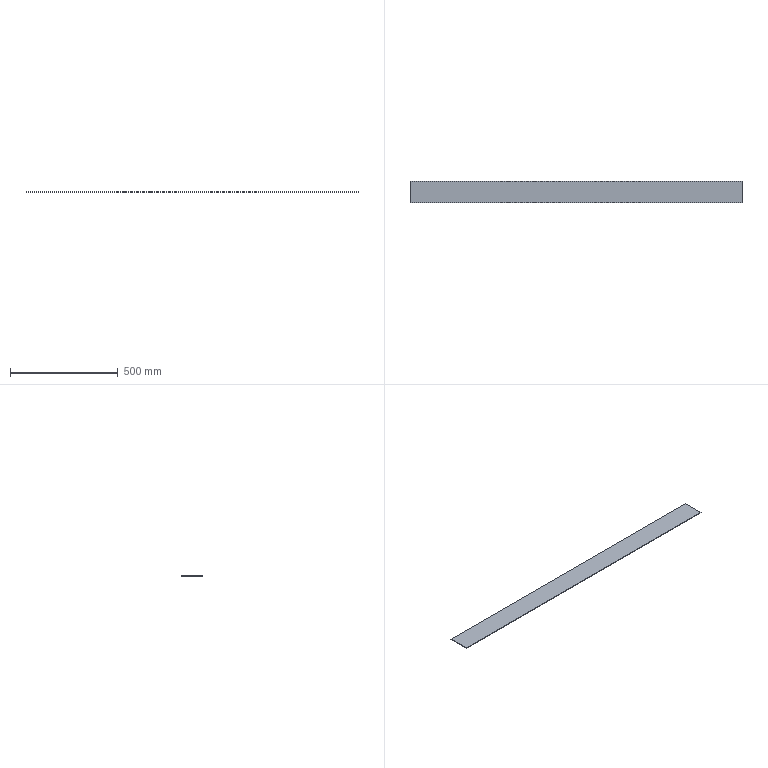Part | STEP file | Double-tube top cross plate SGN-1-03 | 1 solid | 6 faces | box 1540 x 100 x 3 mm | volume 462000 mm3 | plane 6
STEP:
#1=CARTESIAN_POINT('',(0.,0.,0.));
#2=DIRECTION('',(0.,0.,1.));
#3=DIRECTION('',(1.,0.,0.));
#4=AXIS2_PLACEMENT_3D('',#1,#2,#3);
#5=CARTESIAN_POINT('',(770.,-50.,0.));
#6=VERTEX_POINT('',#5);
#7=CARTESIAN_POINT('',(770.,50.,0.));
#8=VERTEX_POINT('',#7);
#9=CARTESIAN_POINT('',(770.,-50.,0.));
#10=DIRECTION('',(0.,1.,0.));
#11=VECTOR('',#10,1.);
#12=LINE('',#9,#11);
#13=CARTESIAN_POINT('',(770.,-50.,-3.));
#14=DIRECTION('',(1.,0.,0.));
#15=DIRECTION('',(0.,0.,-1.));
#16=AXIS2_PLACEMENT_3D('',#13,#14,#15);
#17=PLANE('',#16);
#18=CARTESIAN_POINT('',(-3.,0.));
#19=DIRECTION('',(0.,1.));
#20=VECTOR('',#19,1.);
#21=LINE('',#18,#20);
#22=(GEOMETRIC_REPRESENTATION_CONTEXT(2)PARAMETRIC_REPRESENTATION_CONTEXT()REPRESENTATION_CONTEXT('',''));
#23=DEFINITIONAL_REPRESENTATION('',(#21),#22);
#24=PCURVE('',#17,#23);
#25=CARTESIAN_POINT('',(0.,0.,0.));
#26=DIRECTION('',(0.,0.,-1.));
#27=DIRECTION('',(-1.,0.,0.));
#28=AXIS2_PLACEMENT_3D('',#25,#26,#27);
#29=PLANE('',#28);
#30=CARTESIAN_POINT('',(-770.,-50.));
#31=DIRECTION('',(0.,1.));
#32=VECTOR('',#31,1.);
#33=LINE('',#30,#32);
#34=(GEOMETRIC_REPRESENTATION_CONTEXT(2)PARAMETRIC_REPRESENTATION_CONTEXT()REPRESENTATION_CONTEXT('',''));
#35=DEFINITIONAL_REPRESENTATION('',(#33),#34);
#36=PCURVE('',#29,#35);
#37=SURFACE_CURVE('',#12,(#24,#36),.PCURVE_S1.);
#38=EDGE_CURVE('',#6,#8,#37,.T.);
#39=ORIENTED_EDGE('',*,*,#38,.F.);
#40=CARTESIAN_POINT('',(770.,-50.,-3.));
#41=VERTEX_POINT('',#40);
#42=CARTESIAN_POINT('',(770.,-50.,-3.));
#43=DIRECTION('',(0.,0.,1.));
#44=VECTOR('',#43,1.);
#45=LINE('',#42,#44);
#46=CARTESIAN_POINT('',(0.,0.));
#47=DIRECTION('',(-1.,0.));
#48=VECTOR('',#47,1.);
#49=LINE('',#46,#48);
#50=(GEOMETRIC_REPRESENTATION_CONTEXT(2)PARAMETRIC_REPRESENTATION_CONTEXT()REPRESENTATION_CONTEXT('',''));
#51=DEFINITIONAL_REPRESENTATION('',(#49),#50);
#52=PCURVE('',#17,#51);
#53=CARTESIAN_POINT('',(-770.,-50.,-3.));
#54=DIRECTION('',(0.,-1.,0.));
#55=DIRECTION('',(0.,0.,-1.));
#56=AXIS2_PLACEMENT_3D('',#53,#54,#55);
#57=PLANE('',#56);
#58=CARTESIAN_POINT('',(0.,1540.));
#59=DIRECTION('',(-1.,0.));
#60=VECTOR('',#59,1.);
#61=LINE('',#58,#60);
#62=(GEOMETRIC_REPRESENTATION_CONTEXT(2)PARAMETRIC_REPRESENTATION_CONTEXT()REPRESENTATION_CONTEXT('',''));
#63=DEFINITIONAL_REPRESENTATION('',(#61),#62);
#64=PCURVE('',#57,#63);
#65=SURFACE_CURVE('',#45,(#52,#64),.PCURVE_S1.);
#66=EDGE_CURVE('',#41,#6,#65,.T.);
#67=ORIENTED_EDGE('',*,*,#66,.F.);
#68=CARTESIAN_POINT('',(770.,50.,-3.));
#69=VERTEX_POINT('',#68);
#70=CARTESIAN_POINT('',(770.,-50.,-3.));
#71=DIRECTION('',(0.,1.,0.));
#72=VECTOR('',#71,1.);
#73=LINE('',#70,#72);
#74=CARTESIAN_POINT('',(0.,0.));
#75=DIRECTION('',(0.,1.));
#76=VECTOR('',#75,1.);
#77=LINE('',#74,#76);
#78=(GEOMETRIC_REPRESENTATION_CONTEXT(2)PARAMETRIC_REPRESENTATION_CONTEXT()REPRESENTATION_CONTEXT('',''));
#79=DEFINITIONAL_REPRESENTATION('',(#77),#78);
#80=PCURVE('',#17,#79);
#81=CARTESIAN_POINT('',(0.,0.,-3.));
#82=DIRECTION('',(0.,0.,-1.));
#83=DIRECTION('',(-1.,0.,0.));
#84=AXIS2_PLACEMENT_3D('',#81,#82,#83);
#85=PLANE('',#84);
#86=CARTESIAN_POINT('',(-770.,-50.));
#87=DIRECTION('',(0.,1.));
#88=VECTOR('',#87,1.);
#89=LINE('',#86,#88);
#90=(GEOMETRIC_REPRESENTATION_CONTEXT(2)PARAMETRIC_REPRESENTATION_CONTEXT()REPRESENTATION_CONTEXT('',''));
#91=DEFINITIONAL_REPRESENTATION('',(#89),#90);
#92=PCURVE('',#85,#91);
#93=SURFACE_CURVE('',#73,(#80,#92),.PCURVE_S1.);
#94=EDGE_CURVE('',#41,#69,#93,.T.);
#95=ORIENTED_EDGE('',*,*,#94,.T.);
#96=CARTESIAN_POINT('',(770.,50.,-3.));
#97=DIRECTION('',(0.,0.,1.));
#98=VECTOR('',#97,1.);
#99=LINE('',#96,#98);
#100=CARTESIAN_POINT('',(0.,100.));
#101=DIRECTION('',(-1.,0.));
#102=VECTOR('',#101,1.);
#103=LINE('',#100,#102);
#104=(GEOMETRIC_REPRESENTATION_CONTEXT(2)PARAMETRIC_REPRESENTATION_CONTEXT()REPRESENTATION_CONTEXT('',''));
#105=DEFINITIONAL_REPRESENTATION('',(#103),#104);
#106=PCURVE('',#17,#105);
#107=CARTESIAN_POINT('',(-770.,50.,-3.));
#108=DIRECTION('',(0.,1.,0.));
#109=DIRECTION('',(0.,0.,1.));
#110=AXIS2_PLACEMENT_3D('',#107,#108,#109);
#111=PLANE('',#110);
#112=CARTESIAN_POINT('',(0.,1540.));
#113=DIRECTION('',(1.,0.));
#114=VECTOR('',#113,1.);
#115=LINE('',#112,#114);
#116=(GEOMETRIC_REPRESENTATION_CONTEXT(2)PARAMETRIC_REPRESENTATION_CONTEXT()REPRESENTATION_CONTEXT('',''));
#117=DEFINITIONAL_REPRESENTATION('',(#115),#116);
#118=PCURVE('',#111,#117);
#119=SURFACE_CURVE('',#99,(#106,#118),.PCURVE_S1.);
#120=EDGE_CURVE('',#69,#8,#119,.T.);
#121=ORIENTED_EDGE('',*,*,#120,.T.);
#122=EDGE_LOOP('',(#39,#67,#95,#121));
#123=FACE_BOUND('',#122,.T.);
#124=ADVANCED_FACE('',(#123),#17,.T.);
#125=CARTESIAN_POINT('',(-770.,-50.,0.));
#126=VERTEX_POINT('',#125);
#127=CARTESIAN_POINT('',(-770.,-50.,0.));
#128=DIRECTION('',(1.,0.,0.));
#129=VECTOR('',#128,1.);
#130=LINE('',#127,#129);
#131=CARTESIAN_POINT('',(-3.,0.));
#132=DIRECTION('',(0.,1.));
#133=VECTOR('',#132,1.);
#134=LINE('',#131,#133);
#135=(GEOMETRIC_REPRESENTATION_CONTEXT(2)PARAMETRIC_REPRESENTATION_CONTEXT()REPRESENTATION_CONTEXT('',''));
#136=DEFINITIONAL_REPRESENTATION('',(#134),#135);
#137=PCURVE('',#57,#136);
#138=CARTESIAN_POINT('',(770.,-50.));
#139=DIRECTION('',(-1.,0.));
#140=VECTOR('',#139,1.);
#141=LINE('',#138,#140);
#142=(GEOMETRIC_REPRESENTATION_CONTEXT(2)PARAMETRIC_REPRESENTATION_CONTEXT()REPRESENTATION_CONTEXT('',''));
#143=DEFINITIONAL_REPRESENTATION('',(#141),#142);
#144=PCURVE('',#29,#143);
#145=SURFACE_CURVE('',#130,(#137,#144),.PCURVE_S1.);
#146=EDGE_CURVE('',#126,#6,#145,.T.);
#147=ORIENTED_EDGE('',*,*,#146,.F.);
#148=CARTESIAN_POINT('',(-770.,-50.,-3.));
#149=VERTEX_POINT('',#148);
#150=CARTESIAN_POINT('',(-770.,-50.,-3.));
#151=DIRECTION('',(0.,0.,1.));
#152=VECTOR('',#151,1.);
#153=LINE('',#150,#152);
#154=CARTESIAN_POINT('',(0.,0.));
#155=DIRECTION('',(-1.,0.));
#156=VECTOR('',#155,1.);
#157=LINE('',#154,#156);
#158=(GEOMETRIC_REPRESENTATION_CONTEXT(2)PARAMETRIC_REPRESENTATION_CONTEXT()REPRESENTATION_CONTEXT('',''));
#159=DEFINITIONAL_REPRESENTATION('',(#157),#158);
#160=PCURVE('',#57,#159);
#161=CARTESIAN_POINT('',(-770.,-50.,-3.));
#162=DIRECTION('',(-1.,0.,0.));
#163=DIRECTION('',(0.,0.,1.));
#164=AXIS2_PLACEMENT_3D('',#161,#162,#163);
#165=PLANE('',#164);
#166=CARTESIAN_POINT('',(0.,0.));
#167=DIRECTION('',(1.,0.));
#168=VECTOR('',#167,1.);
#169=LINE('',#166,#168);
#170=(GEOMETRIC_REPRESENTATION_CONTEXT(2)PARAMETRIC_REPRESENTATION_CONTEXT()REPRESENTATION_CONTEXT('',''));
#171=DEFINITIONAL_REPRESENTATION('',(#169),#170);
#172=PCURVE('',#165,#171);
#173=SURFACE_CURVE('',#153,(#160,#172),.PCURVE_S1.);
#174=EDGE_CURVE('',#149,#126,#173,.T.);
#175=ORIENTED_EDGE('',*,*,#174,.F.);
#176=CARTESIAN_POINT('',(-770.,-50.,-3.));
#177=DIRECTION('',(1.,0.,0.));
#178=VECTOR('',#177,1.);
#179=LINE('',#176,#178);
#180=CARTESIAN_POINT('',(0.,0.));
#181=DIRECTION('',(0.,1.));
#182=VECTOR('',#181,1.);
#183=LINE('',#180,#182);
#184=(GEOMETRIC_REPRESENTATION_CONTEXT(2)PARAMETRIC_REPRESENTATION_CONTEXT()REPRESENTATION_CONTEXT('',''));
#185=DEFINITIONAL_REPRESENTATION('',(#183),#184);
#186=PCURVE('',#57,#185);
#187=CARTESIAN_POINT('',(770.,-50.));
#188=DIRECTION('',(-1.,0.));
#189=VECTOR('',#188,1.);
#190=LINE('',#187,#189);
#191=(GEOMETRIC_REPRESENTATION_CONTEXT(2)PARAMETRIC_REPRESENTATION_CONTEXT()REPRESENTATION_CONTEXT('',''));
#192=DEFINITIONAL_REPRESENTATION('',(#190),#191);
#193=PCURVE('',#85,#192);
#194=SURFACE_CURVE('',#179,(#186,#193),.PCURVE_S1.);
#195=EDGE_CURVE('',#149,#41,#194,.T.);
#196=ORIENTED_EDGE('',*,*,#195,.T.);
#197=ORIENTED_EDGE('',*,*,#66,.T.);
#198=EDGE_LOOP('',(#147,#175,#196,#197));
#199=FACE_BOUND('',#198,.T.);
#200=ADVANCED_FACE('',(#199),#57,.T.);
#201=CARTESIAN_POINT('',(-770.,50.,0.));
#202=VERTEX_POINT('',#201);
#203=CARTESIAN_POINT('',(-770.,-50.,0.));
#204=DIRECTION('',(0.,-1.,0.));
#205=VECTOR('',#204,1.);
#206=LINE('',#203,#205);
#207=CARTESIAN_POINT('',(3.,0.));
#208=DIRECTION('',(0.,-1.));
#209=VECTOR('',#208,1.);
#210=LINE('',#207,#209);
#211=(GEOMETRIC_REPRESENTATION_CONTEXT(2)PARAMETRIC_REPRESENTATION_CONTEXT()REPRESENTATION_CONTEXT('',''));
#212=DEFINITIONAL_REPRESENTATION('',(#210),#211);
#213=PCURVE('',#165,#212);
#214=CARTESIAN_POINT('',(770.,-50.));
#215=DIRECTION('',(0.,-1.));
#216=VECTOR('',#215,1.);
#217=LINE('',#214,#216);
#218=(GEOMETRIC_REPRESENTATION_CONTEXT(2)PARAMETRIC_REPRESENTATION_CONTEXT()REPRESENTATION_CONTEXT('',''));
#219=DEFINITIONAL_REPRESENTATION('',(#217),#218);
#220=PCURVE('',#29,#219);
#221=SURFACE_CURVE('',#206,(#213,#220),.PCURVE_S1.);
#222=EDGE_CURVE('',#202,#126,#221,.T.);
#223=ORIENTED_EDGE('',*,*,#222,.F.);
#224=CARTESIAN_POINT('',(-770.,50.,-3.));
#225=VERTEX_POINT('',#224);
#226=CARTESIAN_POINT('',(-770.,50.,-3.));
#227=DIRECTION('',(0.,0.,1.));
#228=VECTOR('',#227,1.);
#229=LINE('',#226,#228);
#230=CARTESIAN_POINT('',(0.,100.));
#231=DIRECTION('',(1.,0.));
#232=VECTOR('',#231,1.);
#233=LINE('',#230,#232);
#234=(GEOMETRIC_REPRESENTATION_CONTEXT(2)PARAMETRIC_REPRESENTATION_CONTEXT()REPRESENTATION_CONTEXT('',''));
#235=DEFINITIONAL_REPRESENTATION('',(#233),#234);
#236=PCURVE('',#165,#235);
#237=CARTESIAN_POINT('',(0.,0.));
#238=DIRECTION('',(1.,0.));
#239=VECTOR('',#238,1.);
#240=LINE('',#237,#239);
#241=(GEOMETRIC_REPRESENTATION_CONTEXT(2)PARAMETRIC_REPRESENTATION_CONTEXT()REPRESENTATION_CONTEXT('',''));
#242=DEFINITIONAL_REPRESENTATION('',(#240),#241);
#243=PCURVE('',#111,#242);
#244=SURFACE_CURVE('',#229,(#236,#243),.PCURVE_S1.);
#245=EDGE_CURVE('',#225,#202,#244,.T.);
#246=ORIENTED_EDGE('',*,*,#245,.F.);
#247=CARTESIAN_POINT('',(-770.,-50.,-3.));
#248=DIRECTION('',(0.,-1.,0.));
#249=VECTOR('',#248,1.);
#250=LINE('',#247,#249);
#251=CARTESIAN_POINT('',(0.,0.));
#252=DIRECTION('',(0.,-1.));
#253=VECTOR('',#252,1.);
#254=LINE('',#251,#253);
#255=(GEOMETRIC_REPRESENTATION_CONTEXT(2)PARAMETRIC_REPRESENTATION_CONTEXT()REPRESENTATION_CONTEXT('',''));
#256=DEFINITIONAL_REPRESENTATION('',(#254),#255);
#257=PCURVE('',#165,#256);
#258=CARTESIAN_POINT('',(770.,-50.));
#259=DIRECTION('',(0.,-1.));
#260=VECTOR('',#259,1.);
#261=LINE('',#258,#260);
#262=(GEOMETRIC_REPRESENTATION_CONTEXT(2)PARAMETRIC_REPRESENTATION_CONTEXT()REPRESENTATION_CONTEXT('',''));
#263=DEFINITIONAL_REPRESENTATION('',(#261),#262);
#264=PCURVE('',#85,#263);
#265=SURFACE_CURVE('',#250,(#257,#264),.PCURVE_S1.);
#266=EDGE_CURVE('',#225,#149,#265,.T.);
#267=ORIENTED_EDGE('',*,*,#266,.T.);
#268=ORIENTED_EDGE('',*,*,#174,.T.);
#269=EDGE_LOOP('',(#223,#246,#267,#268));
#270=FACE_BOUND('',#269,.T.);
#271=ADVANCED_FACE('',(#270),#165,.T.);
#272=CARTESIAN_POINT('',(-770.,50.,0.));
#273=DIRECTION('',(-1.,0.,0.));
#274=VECTOR('',#273,1.);
#275=LINE('',#272,#274);
#276=CARTESIAN_POINT('',(3.,0.));
#277=DIRECTION('',(0.,-1.));
#278=VECTOR('',#277,1.);
#279=LINE('',#276,#278);
#280=(GEOMETRIC_REPRESENTATION_CONTEXT(2)PARAMETRIC_REPRESENTATION_CONTEXT()REPRESENTATION_CONTEXT('',''));
#281=DEFINITIONAL_REPRESENTATION('',(#279),#280);
#282=PCURVE('',#111,#281);
#283=CARTESIAN_POINT('',(770.,50.));
#284=DIRECTION('',(1.,0.));
#285=VECTOR('',#284,1.);
#286=LINE('',#283,#285);
#287=(GEOMETRIC_REPRESENTATION_CONTEXT(2)PARAMETRIC_REPRESENTATION_CONTEXT()REPRESENTATION_CONTEXT('',''));
#288=DEFINITIONAL_REPRESENTATION('',(#286),#287);
#289=PCURVE('',#29,#288);
#290=SURFACE_CURVE('',#275,(#282,#289),.PCURVE_S1.);
#291=EDGE_CURVE('',#8,#202,#290,.T.);
#292=ORIENTED_EDGE('',*,*,#291,.F.);
#293=ORIENTED_EDGE('',*,*,#120,.F.);
#294=CARTESIAN_POINT('',(-770.,50.,-3.));
#295=DIRECTION('',(-1.,0.,0.));
#296=VECTOR('',#295,1.);
#297=LINE('',#294,#296);
#298=CARTESIAN_POINT('',(0.,0.));
#299=DIRECTION('',(0.,-1.));
#300=VECTOR('',#299,1.);
#301=LINE('',#298,#300);
#302=(GEOMETRIC_REPRESENTATION_CONTEXT(2)PARAMETRIC_REPRESENTATION_CONTEXT()REPRESENTATION_CONTEXT('',''));
#303=DEFINITIONAL_REPRESENTATION('',(#301),#302);
#304=PCURVE('',#111,#303);
#305=CARTESIAN_POINT('',(770.,50.));
#306=DIRECTION('',(1.,0.));
#307=VECTOR('',#306,1.);
#308=LINE('',#305,#307);
#309=(GEOMETRIC_REPRESENTATION_CONTEXT(2)PARAMETRIC_REPRESENTATION_CONTEXT()REPRESENTATION_CONTEXT('',''));
#310=DEFINITIONAL_REPRESENTATION('',(#308),#309);
#311=PCURVE('',#85,#310);
#312=SURFACE_CURVE('',#297,(#304,#311),.PCURVE_S1.);
#313=EDGE_CURVE('',#69,#225,#312,.T.);
#314=ORIENTED_EDGE('',*,*,#313,.T.);
#315=ORIENTED_EDGE('',*,*,#245,.T.);
#316=EDGE_LOOP('',(#292,#293,#314,#315));
#317=FACE_BOUND('',#316,.T.);
#318=ADVANCED_FACE('',(#317),#111,.T.);
#319=ORIENTED_EDGE('',*,*,#94,.F.);
#320=ORIENTED_EDGE('',*,*,#195,.F.);
#321=ORIENTED_EDGE('',*,*,#266,.F.);
#322=ORIENTED_EDGE('',*,*,#313,.F.);
#323=EDGE_LOOP('',(#319,#320,#321,#322));
#324=FACE_BOUND('',#323,.T.);
#325=ADVANCED_FACE('',(#324),#85,.T.);
#326=ORIENTED_EDGE('',*,*,#38,.T.);
#327=ORIENTED_EDGE('',*,*,#291,.T.);
#328=ORIENTED_EDGE('',*,*,#222,.T.);
#329=ORIENTED_EDGE('',*,*,#146,.T.);
#330=EDGE_LOOP('',(#326,#327,#328,#329));
#331=FACE_BOUND('',#330,.T.);
#332=ADVANCED_FACE('',(#331),#29,.F.);
#333=CLOSED_SHELL('',(#124,#200,#271,#318,#325,#332));
#334=MANIFOLD_SOLID_BREP('',#333);
#335=(LENGTH_UNIT()NAMED_UNIT(*)SI_UNIT(.MILLI.,.METRE.));
#336=UNCERTAINTY_MEASURE_WITH_UNIT(LENGTH_MEASURE(0.0000001),#335,'','');
#337=(NAMED_UNIT(*)PLANE_ANGLE_UNIT()SI_UNIT($,.RADIAN.));
#338=(NAMED_UNIT(*)SI_UNIT($,.STERADIAN.)SOLID_ANGLE_UNIT());
#339=(GEOMETRIC_REPRESENTATION_CONTEXT(3)GLOBAL_UNCERTAINTY_ASSIGNED_CONTEXT((#336))GLOBAL_UNIT_ASSIGNED_CONTEXT((#335,#337,#338))REPRESENTATION_CONTEXT('',''));
#340=ADVANCED_BREP_SHAPE_REPRESENTATION('',(#4,#334),#339);